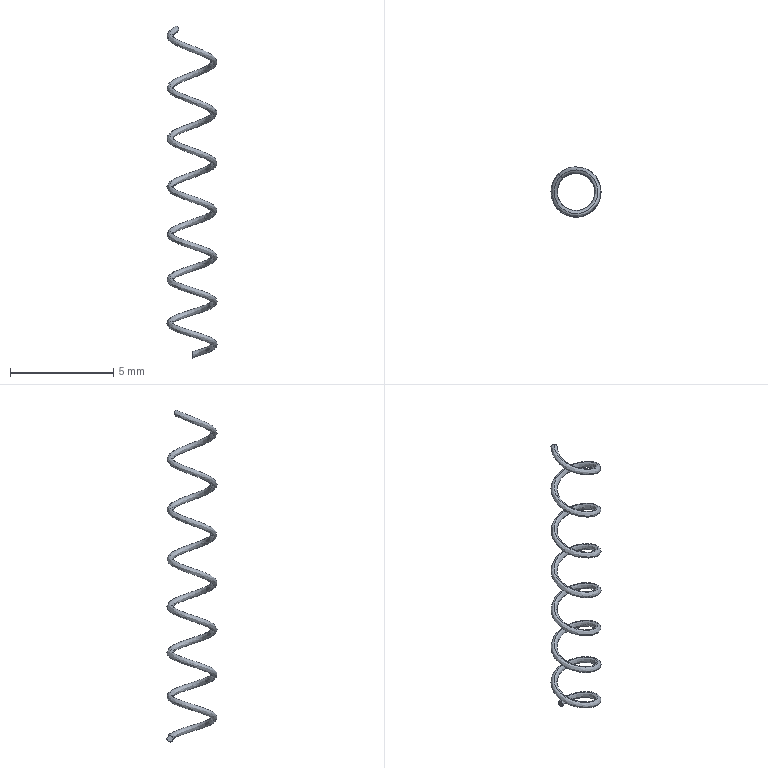Part | SolidWorks | features Helix 1, Sweep 1 | 1 solid | 4 faces | box 2.421 x 2.421 x 16.049 mm | volume 3.23 mm3 | spline 2 | plane 2